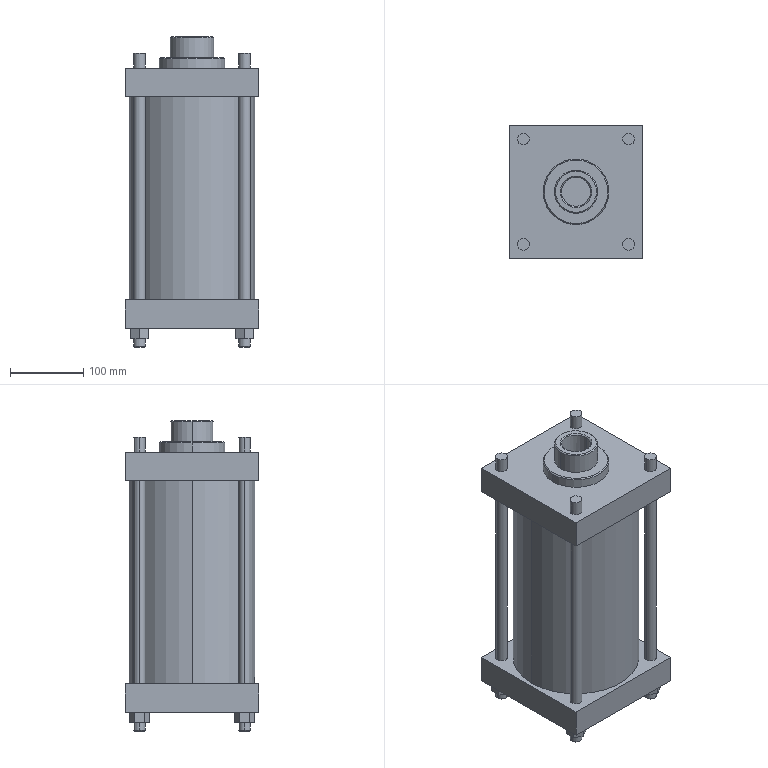Part | STEP file | CDS1FN160-250-A54Z_CS1-Body-1 | 1 solid | 129 faces | box 182 x 182 x 425 mm | volume 4151915 mm3 | plane 63 | cylinder 48 | cone 18 | commonest cylinder face diameters 16 x24 10.3 x6 17.7 x4 26.4 x4 40 x2 59 x2